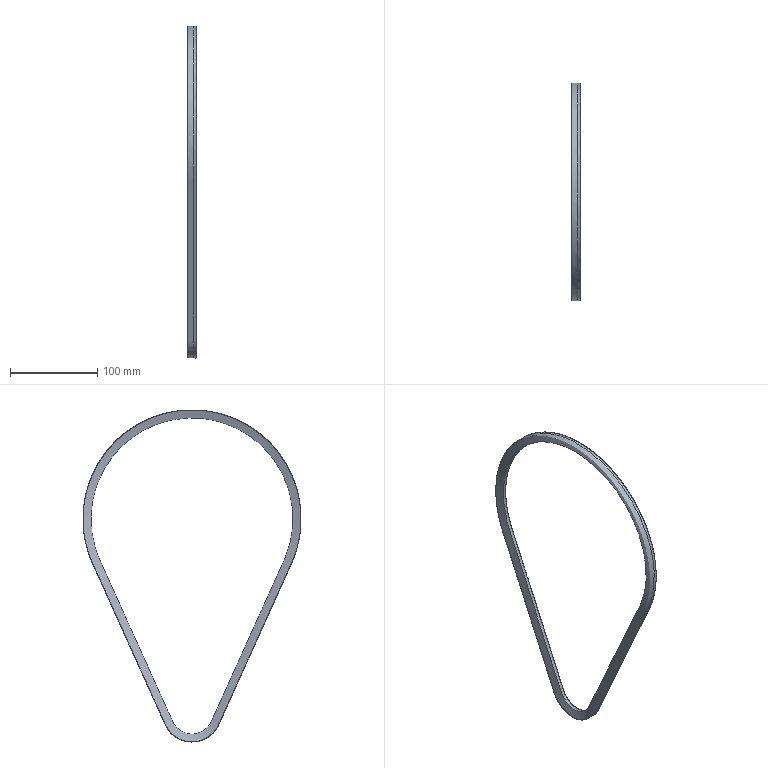Part | NX | features DATUM_CSYS 2, SKETCH 2, DATUM_ON_PATH 1, SKIN 1 | 1 solid | 2 faces | box 10.196 x 249.988 x 380.986 mm | volume 61835 mm3 | spline 2